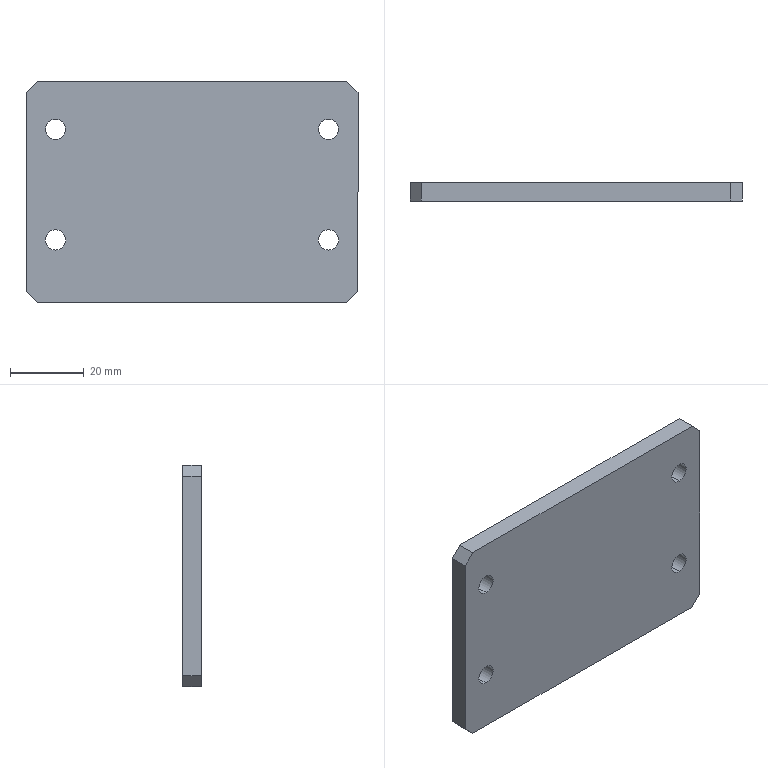Part | SolidWorks | features Chamfer 1, Cut 1, Extrusion 1 | 1 solid | 18 faces | box 90 x 5 x 60 mm | volume 26435 mm3 | plane 10 | cylinder 8 | commonest cylinder face diameters 5.5 x8
STEP:
#1=CARTESIAN_POINT('',(-37.,0.,14.25));
#2=VERTEX_POINT('',#1);
#3=CARTESIAN_POINT('',(-37.,0.,19.75));
#4=VERTEX_POINT('',#3);
#5=CARTESIAN_POINT('',(-37.,0.,17.));
#6=DIRECTION('',(0.,1.,0.));
#7=DIRECTION('',(0.,0.,1.));
#8=AXIS2_PLACEMENT_3D('',#5,#6,#7);
#9=CIRCLE('',#8,2.75);
#10=EDGE_CURVE('',#2,#4,#9,.T.);
#11=ORIENTED_EDGE('',*,*,#10,.F.);
#12=CARTESIAN_POINT('',(-37.,5.,14.25));
#13=VERTEX_POINT('',#12);
#14=CARTESIAN_POINT('',(-37.,-5.,14.25));
#15=DIRECTION('',(0.,1.,0.));
#16=VECTOR('',#15,1000.);
#17=LINE('',#14,#16);
#18=EDGE_CURVE('',#2,#13,#17,.T.);
#19=ORIENTED_EDGE('',*,*,#18,.T.);
#20=CARTESIAN_POINT('',(-37.,5.,19.75));
#21=VERTEX_POINT('',#20);
#22=CARTESIAN_POINT('',(-37.,5.,17.));
#23=DIRECTION('',(0.,1.,0.));
#24=DIRECTION('',(0.,0.,1.));
#25=AXIS2_PLACEMENT_3D('',#22,#23,#24);
#26=CIRCLE('',#25,2.75);
#27=EDGE_CURVE('',#13,#21,#26,.T.);
#28=ORIENTED_EDGE('',*,*,#27,.T.);
#29=CARTESIAN_POINT('',(-37.,-5.,19.75));
#30=DIRECTION('',(0.,1.,0.));
#31=VECTOR('',#30,1000.);
#32=LINE('',#29,#31);
#33=EDGE_CURVE('',#4,#21,#32,.T.);
#34=ORIENTED_EDGE('',*,*,#33,.F.);
#35=EDGE_LOOP('',(#11,#19,#28,#34));
#36=FACE_OUTER_BOUND('',#35,.T.);
#37=CARTESIAN_POINT('',(-37.,-5.,17.));
#38=DIRECTION('',(0.,1.,0.));
#39=DIRECTION('',(0.,0.,1.));
#40=AXIS2_PLACEMENT_3D('',#37,#38,#39);
#41=CYLINDRICAL_SURFACE('',#40,2.75);
#42=ADVANCED_FACE('',(#36),#41,.F.);
#43=CARTESIAN_POINT('',(37.,0.,-15.75));
#44=VERTEX_POINT('',#43);
#45=CARTESIAN_POINT('',(37.,0.,-10.25));
#46=VERTEX_POINT('',#45);
#47=CARTESIAN_POINT('',(37.,0.,-13.));
#48=DIRECTION('',(0.,1.,0.));
#49=DIRECTION('',(0.,0.,1.));
#50=AXIS2_PLACEMENT_3D('',#47,#48,#49);
#51=CIRCLE('',#50,2.75);
#52=EDGE_CURVE('',#44,#46,#51,.T.);
#53=ORIENTED_EDGE('',*,*,#52,.F.);
#54=CARTESIAN_POINT('',(37.,5.,-15.75));
#55=VERTEX_POINT('',#54);
#56=CARTESIAN_POINT('',(37.,-5.,-15.75));
#57=DIRECTION('',(0.,1.,0.));
#58=VECTOR('',#57,1000.);
#59=LINE('',#56,#58);
#60=EDGE_CURVE('',#44,#55,#59,.T.);
#61=ORIENTED_EDGE('',*,*,#60,.T.);
#62=CARTESIAN_POINT('',(37.,5.,-10.25));
#63=VERTEX_POINT('',#62);
#64=CARTESIAN_POINT('',(37.,5.,-13.));
#65=DIRECTION('',(0.,1.,0.));
#66=DIRECTION('',(0.,0.,1.));
#67=AXIS2_PLACEMENT_3D('',#64,#65,#66);
#68=CIRCLE('',#67,2.75);
#69=EDGE_CURVE('',#55,#63,#68,.T.);
#70=ORIENTED_EDGE('',*,*,#69,.T.);
#71=CARTESIAN_POINT('',(37.,-5.,-10.25));
#72=DIRECTION('',(0.,1.,0.));
#73=VECTOR('',#72,1000.);
#74=LINE('',#71,#73);
#75=EDGE_CURVE('',#46,#63,#74,.T.);
#76=ORIENTED_EDGE('',*,*,#75,.F.);
#77=EDGE_LOOP('',(#53,#61,#70,#76));
#78=FACE_OUTER_BOUND('',#77,.T.);
#79=CARTESIAN_POINT('',(37.,-5.,-13.));
#80=DIRECTION('',(0.,1.,0.));
#81=DIRECTION('',(0.,0.,1.));
#82=AXIS2_PLACEMENT_3D('',#79,#80,#81);
#83=CYLINDRICAL_SURFACE('',#82,2.75);
#84=ADVANCED_FACE('',(#78),#83,.F.);
#85=CARTESIAN_POINT('',(-37.,0.,-15.75));
#86=VERTEX_POINT('',#85);
#87=CARTESIAN_POINT('',(-37.,0.,-10.25));
#88=VERTEX_POINT('',#87);
#89=CARTESIAN_POINT('',(-37.,0.,-13.));
#90=DIRECTION('',(0.,1.,0.));
#91=DIRECTION('',(0.,0.,1.));
#92=AXIS2_PLACEMENT_3D('',#89,#90,#91);
#93=CIRCLE('',#92,2.75);
#94=EDGE_CURVE('',#86,#88,#93,.T.);
#95=ORIENTED_EDGE('',*,*,#94,.F.);
#96=CARTESIAN_POINT('',(-37.,5.,-15.75));
#97=VERTEX_POINT('',#96);
#98=CARTESIAN_POINT('',(-37.,-5.,-15.75));
#99=DIRECTION('',(0.,1.,0.));
#100=VECTOR('',#99,1000.);
#101=LINE('',#98,#100);
#102=EDGE_CURVE('',#86,#97,#101,.T.);
#103=ORIENTED_EDGE('',*,*,#102,.T.);
#104=CARTESIAN_POINT('',(-37.,5.,-10.25));
#105=VERTEX_POINT('',#104);
#106=CARTESIAN_POINT('',(-37.,5.,-13.));
#107=DIRECTION('',(0.,1.,0.));
#108=DIRECTION('',(0.,0.,1.));
#109=AXIS2_PLACEMENT_3D('',#106,#107,#108);
#110=CIRCLE('',#109,2.75);
#111=EDGE_CURVE('',#97,#105,#110,.T.);
#112=ORIENTED_EDGE('',*,*,#111,.T.);
#113=CARTESIAN_POINT('',(-37.,-5.,-10.25));
#114=DIRECTION('',(0.,1.,0.));
#115=VECTOR('',#114,1000.);
#116=LINE('',#113,#115);
#117=EDGE_CURVE('',#88,#105,#116,.T.);
#118=ORIENTED_EDGE('',*,*,#117,.F.);
#119=EDGE_LOOP('',(#95,#103,#112,#118));
#120=FACE_OUTER_BOUND('',#119,.T.);
#121=CARTESIAN_POINT('',(-37.,-5.,-13.));
#122=DIRECTION('',(0.,1.,0.));
#123=DIRECTION('',(0.,0.,1.));
#124=AXIS2_PLACEMENT_3D('',#121,#122,#123);
#125=CYLINDRICAL_SURFACE('',#124,2.75);
#126=ADVANCED_FACE('',(#120),#125,.F.);
#127=CARTESIAN_POINT('',(37.,0.,14.25));
#128=VERTEX_POINT('',#127);
#129=CARTESIAN_POINT('',(37.,0.,19.75));
#130=VERTEX_POINT('',#129);
#131=CARTESIAN_POINT('',(37.,0.,17.));
#132=DIRECTION('',(0.,1.,0.));
#133=DIRECTION('',(0.,0.,1.));
#134=AXIS2_PLACEMENT_3D('',#131,#132,#133);
#135=CIRCLE('',#134,2.75);
#136=EDGE_CURVE('',#128,#130,#135,.T.);
#137=ORIENTED_EDGE('',*,*,#136,.F.);
#138=CARTESIAN_POINT('',(37.,5.,14.25));
#139=VERTEX_POINT('',#138);
#140=CARTESIAN_POINT('',(37.,-5.,14.25));
#141=DIRECTION('',(0.,1.,0.));
#142=VECTOR('',#141,1000.);
#143=LINE('',#140,#142);
#144=EDGE_CURVE('',#128,#139,#143,.T.);
#145=ORIENTED_EDGE('',*,*,#144,.T.);
#146=CARTESIAN_POINT('',(37.,5.,19.75));
#147=VERTEX_POINT('',#146);
#148=CARTESIAN_POINT('',(37.,5.,17.));
#149=DIRECTION('',(0.,1.,0.));
#150=DIRECTION('',(0.,0.,1.));
#151=AXIS2_PLACEMENT_3D('',#148,#149,#150);
#152=CIRCLE('',#151,2.75);
#153=EDGE_CURVE('',#139,#147,#152,.T.);
#154=ORIENTED_EDGE('',*,*,#153,.T.);
#155=CARTESIAN_POINT('',(37.,-5.,19.75));
#156=DIRECTION('',(0.,1.,0.));
#157=VECTOR('',#156,1000.);
#158=LINE('',#155,#157);
#159=EDGE_CURVE('',#130,#147,#158,.T.);
#160=ORIENTED_EDGE('',*,*,#159,.F.);
#161=EDGE_LOOP('',(#137,#145,#154,#160));
#162=FACE_OUTER_BOUND('',#161,.T.);
#163=CARTESIAN_POINT('',(37.,-5.,17.));
#164=DIRECTION('',(0.,1.,0.));
#165=DIRECTION('',(0.,0.,1.));
#166=AXIS2_PLACEMENT_3D('',#163,#164,#165);
#167=CYLINDRICAL_SURFACE('',#166,2.75);
#168=ADVANCED_FACE('',(#162),#167,.F.);
#169=CARTESIAN_POINT('',(45.,0.,27.));
#170=VERTEX_POINT('',#169);
#171=CARTESIAN_POINT('',(45.,0.,-27.));
#172=VERTEX_POINT('',#171);
#173=CARTESIAN_POINT('',(45.,0.,-30.));
#174=DIRECTION('',(0.,0.,-1.));
#175=VECTOR('',#174,1000.);
#176=LINE('',#173,#175);
#177=EDGE_CURVE('',#170,#172,#176,.T.);
#178=ORIENTED_EDGE('',*,*,#177,.T.);
#179=CARTESIAN_POINT('',(45.,5.,-27.));
#180=VERTEX_POINT('',#179);
#181=CARTESIAN_POINT('',(45.,5.,-27.));
#182=DIRECTION('',(0.,1.,0.));
#183=VECTOR('',#182,1000.);
#184=LINE('',#181,#183);
#185=EDGE_CURVE('',#172,#180,#184,.T.);
#186=ORIENTED_EDGE('',*,*,#185,.T.);
#187=CARTESIAN_POINT('',(45.,5.,27.));
#188=VERTEX_POINT('',#187);
#189=CARTESIAN_POINT('',(45.,5.,-30.));
#190=DIRECTION('',(0.,0.,-1.));
#191=VECTOR('',#190,1000.);
#192=LINE('',#189,#191);
#193=EDGE_CURVE('',#188,#180,#192,.T.);
#194=ORIENTED_EDGE('',*,*,#193,.F.);
#195=CARTESIAN_POINT('',(45.,5.,27.));
#196=DIRECTION('',(0.,-1.,0.));
#197=VECTOR('',#196,1000.);
#198=LINE('',#195,#197);
#199=EDGE_CURVE('',#188,#170,#198,.T.);
#200=ORIENTED_EDGE('',*,*,#199,.T.);
#201=EDGE_LOOP('',(#178,#186,#194,#200));
#202=FACE_OUTER_BOUND('',#201,.T.);
#203=CARTESIAN_POINT('',(45.,5.,-30.));
#204=DIRECTION('',(-1.,0.,0.));
#205=DIRECTION('',(0.,0.,1.));
#206=AXIS2_PLACEMENT_3D('',#203,#204,#205);
#207=PLANE('',#206);
#208=ADVANCED_FACE('',(#202),#207,.F.);
#209=CARTESIAN_POINT('',(42.,0.,-30.));
#210=VERTEX_POINT('',#209);
#211=CARTESIAN_POINT('',(-42.,0.,-30.));
#212=VERTEX_POINT('',#211);
#213=CARTESIAN_POINT('',(-45.,0.,-30.));
#214=DIRECTION('',(-1.,0.,0.));
#215=VECTOR('',#214,1000.);
#216=LINE('',#213,#215);
#217=EDGE_CURVE('',#210,#212,#216,.T.);
#218=ORIENTED_EDGE('',*,*,#217,.T.);
#219=CARTESIAN_POINT('',(-42.,5.,-30.));
#220=VERTEX_POINT('',#219);
#221=CARTESIAN_POINT('',(-42.,5.,-30.));
#222=DIRECTION('',(0.,1.,0.));
#223=VECTOR('',#222,1000.);
#224=LINE('',#221,#223);
#225=EDGE_CURVE('',#212,#220,#224,.T.);
#226=ORIENTED_EDGE('',*,*,#225,.T.);
#227=CARTESIAN_POINT('',(42.,5.,-30.));
#228=VERTEX_POINT('',#227);
#229=CARTESIAN_POINT('',(-45.,5.,-30.));
#230=DIRECTION('',(-1.,0.,0.));
#231=VECTOR('',#230,1000.);
#232=LINE('',#229,#231);
#233=EDGE_CURVE('',#228,#220,#232,.T.);
#234=ORIENTED_EDGE('',*,*,#233,.F.);
#235=CARTESIAN_POINT('',(42.,5.,-30.));
#236=DIRECTION('',(0.,-1.,0.));
#237=VECTOR('',#236,1000.);
#238=LINE('',#235,#237);
#239=EDGE_CURVE('',#228,#210,#238,.T.);
#240=ORIENTED_EDGE('',*,*,#239,.T.);
#241=EDGE_LOOP('',(#218,#226,#234,#240));
#242=FACE_OUTER_BOUND('',#241,.T.);
#243=CARTESIAN_POINT('',(-45.,5.,-30.));
#244=DIRECTION('',(0.,0.,1.));
#245=DIRECTION('',(1.,0.,0.));
#246=AXIS2_PLACEMENT_3D('',#243,#244,#245);
#247=PLANE('',#246);
#248=ADVANCED_FACE('',(#242),#247,.F.);
#249=CARTESIAN_POINT('',(-45.,5.,-27.));
#250=VERTEX_POINT('',#249);
#251=CARTESIAN_POINT('',(-45.,5.,27.));
#252=VERTEX_POINT('',#251);
#253=CARTESIAN_POINT('',(-45.,5.,-30.));
#254=DIRECTION('',(0.,0.,1.));
#255=VECTOR('',#254,1000.);
#256=LINE('',#253,#255);
#257=EDGE_CURVE('',#250,#252,#256,.T.);
#258=ORIENTED_EDGE('',*,*,#257,.F.);
#259=CARTESIAN_POINT('',(-45.,0.,-27.));
#260=VERTEX_POINT('',#259);
#261=CARTESIAN_POINT('',(-45.,5.,-27.));
#262=DIRECTION('',(0.,-1.,0.));
#263=VECTOR('',#262,1000.);
#264=LINE('',#261,#263);
#265=EDGE_CURVE('',#250,#260,#264,.T.);
#266=ORIENTED_EDGE('',*,*,#265,.T.);
#267=CARTESIAN_POINT('',(-45.,0.,27.));
#268=VERTEX_POINT('',#267);
#269=CARTESIAN_POINT('',(-45.,0.,-30.));
#270=DIRECTION('',(0.,0.,1.));
#271=VECTOR('',#270,1000.);
#272=LINE('',#269,#271);
#273=EDGE_CURVE('',#260,#268,#272,.T.);
#274=ORIENTED_EDGE('',*,*,#273,.T.);
#275=CARTESIAN_POINT('',(-45.,5.,27.));
#276=DIRECTION('',(0.,1.,0.));
#277=VECTOR('',#276,1000.);
#278=LINE('',#275,#277);
#279=EDGE_CURVE('',#268,#252,#278,.T.);
#280=ORIENTED_EDGE('',*,*,#279,.T.);
#281=EDGE_LOOP('',(#258,#266,#274,#280));
#282=FACE_OUTER_BOUND('',#281,.T.);
#283=CARTESIAN_POINT('',(-45.,5.,-30.));
#284=DIRECTION('',(1.,0.,0.));
#285=DIRECTION('',(0.,0.,-1.));
#286=AXIS2_PLACEMENT_3D('',#283,#284,#285);
#287=PLANE('',#286);
#288=ADVANCED_FACE('',(#282),#287,.F.);
#289=CARTESIAN_POINT('',(-42.,0.,30.));
#290=VERTEX_POINT('',#289);
#291=CARTESIAN_POINT('',(42.,0.,30.));
#292=VERTEX_POINT('',#291);
#293=CARTESIAN_POINT('',(-45.,0.,30.));
#294=DIRECTION('',(1.,0.,0.));
#295=VECTOR('',#294,1000.);
#296=LINE('',#293,#295);
#297=EDGE_CURVE('',#290,#292,#296,.T.);
#298=ORIENTED_EDGE('',*,*,#297,.T.);
#299=CARTESIAN_POINT('',(42.,5.,30.));
#300=VERTEX_POINT('',#299);
#301=CARTESIAN_POINT('',(42.,5.,30.));
#302=DIRECTION('',(0.,1.,0.));
#303=VECTOR('',#302,1000.);
#304=LINE('',#301,#303);
#305=EDGE_CURVE('',#292,#300,#304,.T.);
#306=ORIENTED_EDGE('',*,*,#305,.T.);
#307=CARTESIAN_POINT('',(-42.,5.,30.));
#308=VERTEX_POINT('',#307);
#309=CARTESIAN_POINT('',(-45.,5.,30.));
#310=DIRECTION('',(1.,0.,0.));
#311=VECTOR('',#310,1000.);
#312=LINE('',#309,#311);
#313=EDGE_CURVE('',#308,#300,#312,.T.);
#314=ORIENTED_EDGE('',*,*,#313,.F.);
#315=CARTESIAN_POINT('',(-42.,5.,30.));
#316=DIRECTION('',(0.,-1.,0.));
#317=VECTOR('',#316,1000.);
#318=LINE('',#315,#317);
#319=EDGE_CURVE('',#308,#290,#318,.T.);
#320=ORIENTED_EDGE('',*,*,#319,.T.);
#321=EDGE_LOOP('',(#298,#306,#314,#320));
#322=FACE_OUTER_BOUND('',#321,.T.);
#323=CARTESIAN_POINT('',(-45.,5.,30.));
#324=DIRECTION('',(0.,0.,-1.));
#325=DIRECTION('',(-1.,0.,0.));
#326=AXIS2_PLACEMENT_3D('',#323,#324,#325);
#327=PLANE('',#326);
#328=ADVANCED_FACE('',(#322),#327,.F.);
#329=CARTESIAN_POINT('',(-37.,5.,17.));
#330=DIRECTION('',(0.,1.,0.));
#331=DIRECTION('',(0.,0.,1.));
#332=AXIS2_PLACEMENT_3D('',#329,#330,#331);
#333=CIRCLE('',#332,2.75);
#334=EDGE_CURVE('',#21,#13,#333,.T.);
#335=ORIENTED_EDGE('',*,*,#334,.F.);
#336=ORIENTED_EDGE('',*,*,#27,.F.);
#337=EDGE_LOOP('',(#335,#336));
#338=FACE_BOUND('',#337,.T.);
#339=CARTESIAN_POINT('',(37.,5.,-13.));
#340=DIRECTION('',(0.,1.,0.));
#341=DIRECTION('',(0.,0.,1.));
#342=AXIS2_PLACEMENT_3D('',#339,#340,#341);
#343=CIRCLE('',#342,2.75);
#344=EDGE_CURVE('',#63,#55,#343,.T.);
#345=ORIENTED_EDGE('',*,*,#344,.F.);
#346=ORIENTED_EDGE('',*,*,#69,.F.);
#347=EDGE_LOOP('',(#345,#346));
#348=FACE_BOUND('',#347,.T.);
#349=CARTESIAN_POINT('',(-37.,5.,-13.));
#350=DIRECTION('',(0.,1.,0.));
#351=DIRECTION('',(0.,0.,1.));
#352=AXIS2_PLACEMENT_3D('',#349,#350,#351);
#353=CIRCLE('',#352,2.75);
#354=EDGE_CURVE('',#105,#97,#353,.T.);
#355=ORIENTED_EDGE('',*,*,#354,.F.);
#356=ORIENTED_EDGE('',*,*,#111,.F.);
#357=EDGE_LOOP('',(#355,#356));
#358=FACE_BOUND('',#357,.T.);
#359=CARTESIAN_POINT('',(37.,5.,17.));
#360=DIRECTION('',(0.,1.,0.));
#361=DIRECTION('',(0.,0.,1.));
#362=AXIS2_PLACEMENT_3D('',#359,#360,#361);
#363=CIRCLE('',#362,2.75);
#364=EDGE_CURVE('',#147,#139,#363,.T.);
#365=ORIENTED_EDGE('',*,*,#364,.F.);
#366=ORIENTED_EDGE('',*,*,#153,.F.);
#367=EDGE_LOOP('',(#365,#366));
#368=FACE_BOUND('',#367,.T.);
#369=ORIENTED_EDGE('',*,*,#233,.T.);
#370=CARTESIAN_POINT('',(-36.,5.,-36.));
#371=DIRECTION('',(-0.7071,0.,0.7071));
#372=VECTOR('',#371,1000.);
#373=LINE('',#370,#372);
#374=EDGE_CURVE('',#220,#250,#373,.T.);
#375=ORIENTED_EDGE('',*,*,#374,.T.);
#376=ORIENTED_EDGE('',*,*,#257,.T.);
#377=CARTESIAN_POINT('',(-36.,5.,36.));
#378=DIRECTION('',(0.7071,0.,0.7071));
#379=VECTOR('',#378,1000.);
#380=LINE('',#377,#379);
#381=EDGE_CURVE('',#252,#308,#380,.T.);
#382=ORIENTED_EDGE('',*,*,#381,.T.);
#383=ORIENTED_EDGE('',*,*,#313,.T.);
#384=CARTESIAN_POINT('',(36.,5.,36.));
#385=DIRECTION('',(0.7071,0.,-0.7071));
#386=VECTOR('',#385,1000.);
#387=LINE('',#384,#386);
#388=EDGE_CURVE('',#300,#188,#387,.T.);
#389=ORIENTED_EDGE('',*,*,#388,.T.);
#390=ORIENTED_EDGE('',*,*,#193,.T.);
#391=CARTESIAN_POINT('',(36.,5.,-36.));
#392=DIRECTION('',(-0.7071,0.,-0.7071));
#393=VECTOR('',#392,1000.);
#394=LINE('',#391,#393);
#395=EDGE_CURVE('',#180,#228,#394,.T.);
#396=ORIENTED_EDGE('',*,*,#395,.T.);
#397=EDGE_LOOP('',(#369,#375,#376,#382,#383,#389,#390,#396));
#398=FACE_OUTER_BOUND('',#397,.T.);
#399=CARTESIAN_POINT('',(0.,5.,0.));
#400=DIRECTION('',(0.,1.,0.));
#401=DIRECTION('',(0.,0.,1.));
#402=AXIS2_PLACEMENT_3D('',#399,#400,#401);
#403=PLANE('',#402);
#404=ADVANCED_FACE('',(#338,#348,#358,#368,#398),#403,.T.);
#405=CARTESIAN_POINT('',(-37.,0.,17.));
#406=DIRECTION('',(0.,1.,0.));
#407=DIRECTION('',(0.,0.,1.));
#408=AXIS2_PLACEMENT_3D('',#405,#406,#407);
#409=CIRCLE('',#408,2.75);
#410=EDGE_CURVE('',#4,#2,#409,.T.);
#411=ORIENTED_EDGE('',*,*,#410,.T.);
#412=ORIENTED_EDGE('',*,*,#10,.T.);
#413=EDGE_LOOP('',(#411,#412));
#414=FACE_BOUND('',#413,.T.);
#415=CARTESIAN_POINT('',(37.,0.,-13.));
#416=DIRECTION('',(0.,1.,0.));
#417=DIRECTION('',(0.,0.,1.));
#418=AXIS2_PLACEMENT_3D('',#415,#416,#417);
#419=CIRCLE('',#418,2.75);
#420=EDGE_CURVE('',#46,#44,#419,.T.);
#421=ORIENTED_EDGE('',*,*,#420,.T.);
#422=ORIENTED_EDGE('',*,*,#52,.T.);
#423=EDGE_LOOP('',(#421,#422));
#424=FACE_BOUND('',#423,.T.);
#425=CARTESIAN_POINT('',(-37.,0.,-13.));
#426=DIRECTION('',(0.,1.,0.));
#427=DIRECTION('',(0.,0.,1.));
#428=AXIS2_PLACEMENT_3D('',#425,#426,#427);
#429=CIRCLE('',#428,2.75);
#430=EDGE_CURVE('',#88,#86,#429,.T.);
#431=ORIENTED_EDGE('',*,*,#430,.T.);
#432=ORIENTED_EDGE('',*,*,#94,.T.);
#433=EDGE_LOOP('',(#431,#432));
#434=FACE_BOUND('',#433,.T.);
#435=CARTESIAN_POINT('',(37.,0.,17.));
#436=DIRECTION('',(0.,1.,0.));
#437=DIRECTION('',(0.,0.,1.));
#438=AXIS2_PLACEMENT_3D('',#435,#436,#437);
#439=CIRCLE('',#438,2.75);
#440=EDGE_CURVE('',#130,#128,#439,.T.);
#441=ORIENTED_EDGE('',*,*,#440,.T.);
#442=ORIENTED_EDGE('',*,*,#136,.T.);
#443=EDGE_LOOP('',(#441,#442));
#444=FACE_BOUND('',#443,.T.);
#445=ORIENTED_EDGE('',*,*,#273,.F.);
#446=CARTESIAN_POINT('',(-45.,0.,-27.));
#447=DIRECTION('',(0.7071,0.,-0.7071));
#448=VECTOR('',#447,1000.);
#449=LINE('',#446,#448);
#450=EDGE_CURVE('',#260,#212,#449,.T.);
#451=ORIENTED_EDGE('',*,*,#450,.T.);
#452=ORIENTED_EDGE('',*,*,#217,.F.);
#453=CARTESIAN_POINT('',(42.,0.,-30.));
#454=DIRECTION('',(0.7071,0.,0.7071));
#455=VECTOR('',#454,1000.);
#456=LINE('',#453,#455);
#457=EDGE_CURVE('',#210,#172,#456,.T.);
#458=ORIENTED_EDGE('',*,*,#457,.T.);
#459=ORIENTED_EDGE('',*,*,#177,.F.);
#460=CARTESIAN_POINT('',(45.,0.,27.));
#461=DIRECTION('',(-0.7071,0.,0.7071));
#462=VECTOR('',#461,1000.);
#463=LINE('',#460,#462);
#464=EDGE_CURVE('',#170,#292,#463,.T.);
#465=ORIENTED_EDGE('',*,*,#464,.T.);
#466=ORIENTED_EDGE('',*,*,#297,.F.);
#467=CARTESIAN_POINT('',(-42.,0.,30.));
#468=DIRECTION('',(-0.7071,0.,-0.7071));
#469=VECTOR('',#468,1000.);
#470=LINE('',#467,#469);
#471=EDGE_CURVE('',#290,#268,#470,.T.);
#472=ORIENTED_EDGE('',*,*,#471,.T.);
#473=EDGE_LOOP('',(#445,#451,#452,#458,#459,#465,#466,#472));
#474=FACE_OUTER_BOUND('',#473,.T.);
#475=CARTESIAN_POINT('',(0.,0.,0.));
#476=DIRECTION('',(0.,1.,0.));
#477=DIRECTION('',(0.,0.,1.));
#478=AXIS2_PLACEMENT_3D('',#475,#476,#477);
#479=PLANE('',#478);
#480=ADVANCED_FACE('',(#414,#424,#434,#444,#474),#479,.F.);
#481=ORIENTED_EDGE('',*,*,#374,.F.);
#482=ORIENTED_EDGE('',*,*,#225,.F.);
#483=ORIENTED_EDGE('',*,*,#450,.F.);
#484=ORIENTED_EDGE('',*,*,#265,.F.);
#485=EDGE_LOOP('',(#481,#482,#483,#484));
#486=FACE_OUTER_BOUND('',#485,.T.);
#487=CARTESIAN_POINT('',(-45.,5.,-27.));
#488=DIRECTION('',(0.7071,0.,0.7071));
#489=DIRECTION('',(0.,-1.,0.));
#490=AXIS2_PLACEMENT_3D('',#487,#488,#489);
#491=PLANE('',#490);
#492=ADVANCED_FACE('',(#486),#491,.F.);
#493=ORIENTED_EDGE('',*,*,#395,.F.);
#494=ORIENTED_EDGE('',*,*,#185,.F.);
#495=ORIENTED_EDGE('',*,*,#457,.F.);
#496=ORIENTED_EDGE('',*,*,#239,.F.);
#497=EDGE_LOOP('',(#493,#494,#495,#496));
#498=FACE_OUTER_BOUND('',#497,.T.);
#499=CARTESIAN_POINT('',(42.,5.,-30.));
#500=DIRECTION('',(-0.7071,0.,0.7071));
#501=DIRECTION('',(0.,-1.,0.));
#502=AXIS2_PLACEMENT_3D('',#499,#500,#501);
#503=PLANE('',#502);
#504=ADVANCED_FACE('',(#498),#503,.F.);
#505=ORIENTED_EDGE('',*,*,#388,.F.);
#506=ORIENTED_EDGE('',*,*,#305,.F.);
#507=ORIENTED_EDGE('',*,*,#464,.F.);
#508=ORIENTED_EDGE('',*,*,#199,.F.);
#509=EDGE_LOOP('',(#505,#506,#507,#508));
#510=FACE_OUTER_BOUND('',#509,.T.);
#511=CARTESIAN_POINT('',(45.,5.,27.));
#512=DIRECTION('',(-0.7071,0.,-0.7071));
#513=DIRECTION('',(0.,-1.,0.));
#514=AXIS2_PLACEMENT_3D('',#511,#512,#513);
#515=PLANE('',#514);
#516=ADVANCED_FACE('',(#510),#515,.F.);
#517=ORIENTED_EDGE('',*,*,#381,.F.);
#518=ORIENTED_EDGE('',*,*,#279,.F.);
#519=ORIENTED_EDGE('',*,*,#471,.F.);
#520=ORIENTED_EDGE('',*,*,#319,.F.);
#521=EDGE_LOOP('',(#517,#518,#519,#520));
#522=FACE_OUTER_BOUND('',#521,.T.);
#523=CARTESIAN_POINT('',(-42.,5.,30.));
#524=DIRECTION('',(0.7071,0.,-0.7071));
#525=DIRECTION('',(0.,-1.,0.));
#526=AXIS2_PLACEMENT_3D('',#523,#524,#525);
#527=PLANE('',#526);
#528=ADVANCED_FACE('',(#522),#527,.F.);
#529=ORIENTED_EDGE('',*,*,#144,.F.);
#530=ORIENTED_EDGE('',*,*,#440,.F.);
#531=ORIENTED_EDGE('',*,*,#159,.T.);
#532=ORIENTED_EDGE('',*,*,#364,.T.);
#533=EDGE_LOOP('',(#529,#530,#531,#532));
#534=FACE_OUTER_BOUND('',#533,.T.);
#535=CARTESIAN_POINT('',(37.,-5.,17.));
#536=DIRECTION('',(0.,1.,0.));
#537=DIRECTION('',(0.,0.,1.));
#538=AXIS2_PLACEMENT_3D('',#535,#536,#537);
#539=CYLINDRICAL_SURFACE('',#538,2.75);
#540=ADVANCED_FACE('',(#534),#539,.F.);
#541=ORIENTED_EDGE('',*,*,#102,.F.);
#542=ORIENTED_EDGE('',*,*,#430,.F.);
#543=ORIENTED_EDGE('',*,*,#117,.T.);
#544=ORIENTED_EDGE('',*,*,#354,.T.);
#545=EDGE_LOOP('',(#541,#542,#543,#544));
#546=FACE_OUTER_BOUND('',#545,.T.);
#547=CARTESIAN_POINT('',(-37.,-5.,-13.));
#548=DIRECTION('',(0.,1.,0.));
#549=DIRECTION('',(0.,0.,1.));
#550=AXIS2_PLACEMENT_3D('',#547,#548,#549);
#551=CYLINDRICAL_SURFACE('',#550,2.75);
#552=ADVANCED_FACE('',(#546),#551,.F.);
#553=ORIENTED_EDGE('',*,*,#60,.F.);
#554=ORIENTED_EDGE('',*,*,#420,.F.);
#555=ORIENTED_EDGE('',*,*,#75,.T.);
#556=ORIENTED_EDGE('',*,*,#344,.T.);
#557=EDGE_LOOP('',(#553,#554,#555,#556));
#558=FACE_OUTER_BOUND('',#557,.T.);
#559=CARTESIAN_POINT('',(37.,-5.,-13.));
#560=DIRECTION('',(0.,1.,0.));
#561=DIRECTION('',(0.,0.,1.));
#562=AXIS2_PLACEMENT_3D('',#559,#560,#561);
#563=CYLINDRICAL_SURFACE('',#562,2.75);
#564=ADVANCED_FACE('',(#558),#563,.F.);
#565=ORIENTED_EDGE('',*,*,#18,.F.);
#566=ORIENTED_EDGE('',*,*,#410,.F.);
#567=ORIENTED_EDGE('',*,*,#33,.T.);
#568=ORIENTED_EDGE('',*,*,#334,.T.);
#569=EDGE_LOOP('',(#565,#566,#567,#568));
#570=FACE_OUTER_BOUND('',#569,.T.);
#571=CARTESIAN_POINT('',(-37.,-5.,17.));
#572=DIRECTION('',(0.,1.,0.));
#573=DIRECTION('',(0.,0.,1.));
#574=AXIS2_PLACEMENT_3D('',#571,#572,#573);
#575=CYLINDRICAL_SURFACE('',#574,2.75);
#576=ADVANCED_FACE('',(#570),#575,.F.);
#577=CLOSED_SHELL('',(#42,#84,#126,#168,#208,#248,#288,#328,#404,#480,#492,#504,#516,#528,#540,#552,#564,#576));
#578=MANIFOLD_SOLID_BREP('',#577);
#579=CARTESIAN_POINT('',(0.,0.,0.));
#580=DIRECTION('',(0.,0.,1.));
#581=DIRECTION('',(1.,0.,0.));
#582=AXIS2_PLACEMENT_3D('',#579,#580,#581);
#583=(LENGTH_UNIT()NAMED_UNIT(*)SI_UNIT(.MILLI.,.METRE.));
#584=UNCERTAINTY_MEASURE_WITH_UNIT(LENGTH_MEASURE(0.00001),#583,'','');
#585=(NAMED_UNIT(*)PLANE_ANGLE_UNIT()SI_UNIT($,.RADIAN.));
#586=(NAMED_UNIT(*)SI_UNIT($,.STERADIAN.)SOLID_ANGLE_UNIT());
#587=(GEOMETRIC_REPRESENTATION_CONTEXT(3)GLOBAL_UNCERTAINTY_ASSIGNED_CONTEXT((#584))GLOBAL_UNIT_ASSIGNED_CONTEXT((#583,#585,#586))REPRESENTATION_CONTEXT('',''));
#588=ADVANCED_BREP_SHAPE_REPRESENTATION('',(#578,#582),#587);